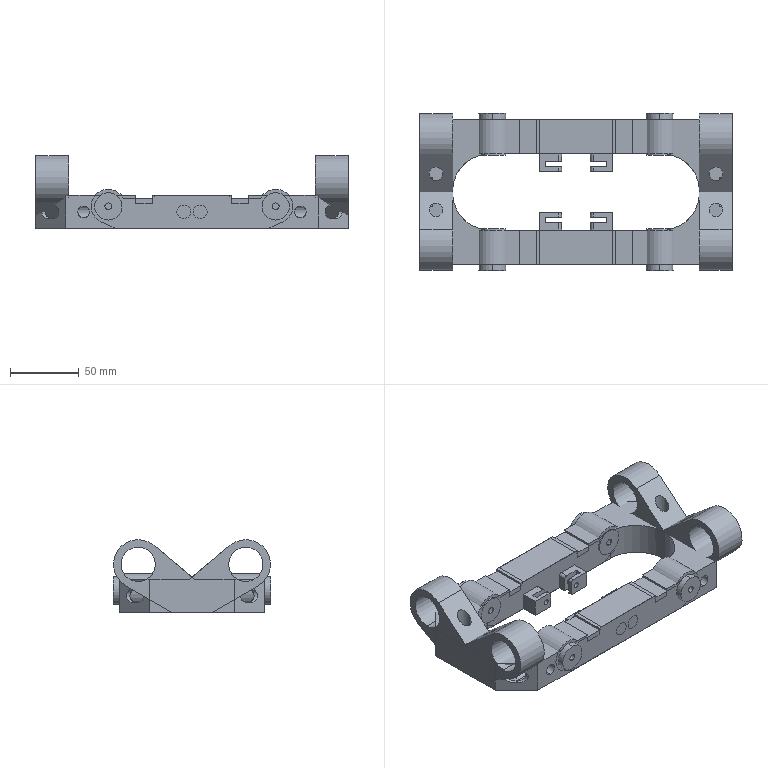NC program | Mastercam | posted with a generic post | part box 228 x 114.503 x 53 mm
Lines 3657 to 5339 of 11407:
(10 BM/BNOS |TOOL - 3|DIA. OFF. - 3|LEN. - 3|TOOL DIA. - 10.)
N7392 T3 M6
N7394 G0 G54 G90 X121.565 Y-17.392 C0. B0. S6000 M3
N7396 G43 H3 Z120.
N7398 Z31.503
N7400 Z28.503
N7402 G1 Z26.503 F600.
N7404 Y-17.366 Z26.183 F1500.
N7406 Y-17.293 Z25.869
N7408 Y-17.179 Z25.562
N7410 Y-17.03 Z25.264
N7412 Y-16.853 Z24.978
N7414 Y-16.654 Z24.707
N7416 Y-16.438 Z24.451
N7418 Y-16.214 Z24.214
N7420 X121.553 Y-16.127 Z24.127
N7422 X121.521 Y-16.044 Z24.044
N7424 X121.468 Y-15.966 Z23.966
N7426 X121.398 Y-15.892 Z23.892
N7428 X121.214 Y-15.757 Z23.757
N7430 X120.982 Y-15.644 Z23.644
N7432 X120.719 Y-15.552 Z23.552
N7434 X120.44 Y-15.484 Z23.484
N7436 X120.162 Y-15.442 Z23.442
N7438 X119.898 Y-15.428 Z23.428
N7440 X119.21
N7442 X118.024
N7444 X116.837
N7446 X115.651
N7448 X114.465
N7450 X113.278
N7452 X112.092
N7454 X110.906
N7456 X109.719
N7458 X108.533
N7460 X107.347
N7462 X106.161
N7464 X104.974
N7466 X103.788
N7468 X102.602
N7470 X101.415
N7472 X100.229
N7474 X99.043
N7476 X97.856
N7478 X96.67
N7480 X95.484
N7482 X94.297
N7484 X93.111
N7486 X91.925
N7488 X90.739
N7490 X89.552
N7492 X88.366
N7494 X87.18
N7496 X85.993
N7498 X84.807
N7500 X83.621
N7502 X82.434
N7504 X81.248
N7506 X80.062
N7508 X78.876
N7510 X77.689
N7512 X76.503
N7514 X75.317
N7516 X74.13
N7518 X72.944
N7520 X71.758
N7522 X70.571
N7524 X69.385
N7526 X68.199
N7528 X67.012
N7530 X65.826
N7532 X64.64
N7534 X63.454
N7536 X62.267
N7538 X61.081
N7540 X59.895
N7542 X58.708
N7544 X57.522
N7546 X56.336
N7548 X55.149
N7550 X53.963
N7552 X52.777
N7554 X51.591
N7556 X50.495 Y-15.429 Z23.442
N7558 X49.466 Y-15.428 Z23.489
N7560 X48.416 Z23.581
N7562 X47.37 Z23.719
N7564 X46.367 Y-15.429 Z23.898
N7566 X45.385 Z24.115
N7568 X44.38 Y-15.428 Z24.387
N7570 X43.376 Z24.707
N7572 X42.385 Z25.069
N7574 X41.432 Y-15.429 Z25.467
N7576 X40.522 Z25.895
N7578 X39.613 Y-15.428 Z26.372
N7580 X38.702 Z26.903
N7582 X37.815 Z27.474
N7584 X36.959 Z28.077
N7586 X36.165 Y-15.429 Z28.694
N7588 X35.393 Y-15.428 Z29.349
N7590 X34.619 Z30.065
N7592 X33.878 Z30.815
N7594 X33.17 Z31.597
N7596 X32.528 Y-15.429 Z32.371
N7598 X31.922 Y-15.428 Z33.173
N7600 X31.323 Z34.041
N7602 X30.762 Z34.934
N7604 X30.243 Z35.852
N7606 X29.783 Y-15.429 Z36.75
N7608 X29.365 Y-15.428 Z37.665
N7610 X28.973 Z38.639
N7612 X28.62 Z39.633
N7614 X28.312 Z40.641
N7616 X28.057 Y-15.429 Z41.633
N7618 X27.848 Z42.616
N7620 X27.679 Y-15.428 Z43.639
N7622 X27.554 Z44.686
N7624 X27.471 Z45.737
N7626 X27.441 Z46.263
N7628 X27.435 Z46.868
N7630 X27.428 Z48.149
N7632 Z49.504
N7634 Z50.86
N7636 Z52.215
N7638 Z53.57
N7640 Z54.925
N7642 Z56.28
N7644 Z57.635
N7646 Z58.99
N7648 Z60.346
N7650 Z61.701
N7652 Z62.378
N7654 X27.434 Y-15.434 Z62.61
N7656 X27.454 Y-15.454 Z62.852
N7658 X27.486 Y-15.486 Z63.101
N7660 X27.529 Y-15.529 Z63.354
N7662 X27.585 Y-15.585 Z63.607
N7664 X27.651 Y-15.651 Z63.856
N7666 X27.729 Y-15.729 Z64.098
N7668 X27.816 Y-15.816 Z64.329
N7670 X27.914 Y-15.914 Z64.546
N7672 X28.021 Y-16.021 Z64.746
N7674 X28.138 Y-16.138 Z64.924
N7676 X28.263 Y-16.263 Z65.078
N7678 X28.396 Y-16.396 Z65.204
N7680 X28.537 Y-16.537 Z65.299
N7682 X28.686 Y-16.686 Z65.358
N7684 X28.842 Y-16.842 Z65.378
N7686 X29.006 Y-17.006 Z65.387
N7688 X29.177 Y-17.177 Z65.415
N7690 X29.353 Y-17.353 Z65.46
N7692 X29.532 Y-17.532 Z65.522
N7694 X29.711 Y-17.711 Z65.6
N7696 X29.887 Y-17.887 Z65.694
N7698 X30.058 Y-18.058 Z65.804
N7700 X30.221 Y-18.221 Z65.928
N7702 X30.375 Y-18.375 Z66.066
N7704 X30.516 Y-18.516 Z66.217
N7706 X30.643 Y-18.643 Z66.382
N7708 X30.751 Y-18.751 Z66.559
N7710 X30.84 Y-18.84 Z66.747
N7712 X30.907 Y-18.907 Z66.947
N7714 X30.949 Y-18.949 Z67.158
N7716 X30.963 Y-18.963 Z67.378
N7718 G0 Z69.378
N7720 Z72.378
N7722 Z120.
N7724 X50. Y16.606
N7726 Z30.273
N7728 Z27.273
N7730 G1 Z25.273 F600.
N7732 Y16.591 Z25.081 F1500.
N7734 Y16.547 Z24.892
N7736 Y16.479 Z24.708
N7738 Y16.389 Z24.53
N7740 Y16.283 Z24.358
N7742 Y16.163 Z24.195
N7744 Y15.899 Z23.899
N7746 X50.027 Y15.798 Z23.798
N7748 X50.1 Y15.706 Z23.706
N7750 X50.211 Y15.626 Z23.626
N7752 X50.35 Y15.557 Z23.557
N7754 X50.508 Y15.502 Z23.502
N7756 X50.675 Y15.462 Z23.462
N7758 X50.842 Y15.437 Z23.437
N7760 X51. Y15.428 Z23.428
N7762 X51.733
N7764 X53.2
N7766 X54.667
N7768 X56.133
N7770 X57.6
N7772 X59.067
N7774 X60.533
N7776 X62.
N7778 X63.467
N7780 X64.933
N7782 X66.4
N7784 X67.867
N7786 X69.333
N7788 X70.8
N7790 X72.267
N7792 X73.
N7794 X73.179 Y15.423
N7796 X73.358 Y15.409
N7798 X73.536 Y15.386
N7800 X73.713 Y15.353
N7802 X73.887 Y15.311
N7804 X74.059 Y15.26
N7806 X74.228 Y15.2
N7808 X74.394 Y15.132
N7810 X74.556 Y15.054
N7812 X74.714 Y14.969
N7814 X74.867 Y14.875
N7816 X75.015 Y14.773
N7818 X75.157 Y14.664
N7820 X75.294 Y14.547
N7822 X75.424 Y14.424
N7824 X75.547 Y14.294
N7826 X75.664 Y14.157
N7828 X75.773 Y14.015
N7830 X75.875 Y13.867
N7832 X75.969 Y13.714
N7834 X76.054 Y13.556
N7836 X76.132 Y13.394
N7838 X76.2 Y13.228
N7840 X76.26 Y13.059
N7842 X76.311 Y12.887
N7844 X76.353 Y12.713
N7846 X76.386 Y12.536
N7848 X76.409 Y12.358
N7850 X76.423 Y12.179
N7852 X76.428 Y12.
N7854 Y11.25
N7856 Y9.75
N7858 Y9.428
N7860 X76.75
N7862 X78.25
N7864 X79.75
N7866 X81.25
N7868 X81.572
N7870 Y9.75
N7872 Y11.25
N7874 Y12.
N7876 X81.577 Y12.179
N7878 X81.591 Y12.358
N7880 X81.614 Y12.536
N7882 X81.647 Y12.713
N7884 X81.689 Y12.887
N7886 X81.74 Y13.059
N7888 X81.8 Y13.228
N7890 X81.868 Y13.394
N7892 X81.946 Y13.556
N7894 X82.031 Y13.714
N7896 X82.125 Y13.867
N7898 X82.227 Y14.015
N7900 X82.336 Y14.157
N7902 X82.453 Y14.294
N7904 X82.576 Y14.424
N7906 X82.706 Y14.547
N7908 X82.843 Y14.664
N7910 X82.985 Y14.773
N7912 X83.133 Y14.875
N7914 X83.286 Y14.969
N7916 X83.444 Y15.054
N7918 X83.606 Y15.132
N7920 X83.772 Y15.2
N7922 X83.941 Y15.26
N7924 X84.113 Y15.311
N7926 X84.287 Y15.353
N7928 X84.464 Y15.386
N7930 X84.642 Y15.409
N7932 X84.821 Y15.423
N7934 X85. Y15.428
N7936 X85.731
N7938 X87.193
N7940 X88.654
N7942 X90.116
N7944 X91.578
N7946 X93.04
N7948 X94.502
N7950 X95.963
N7952 X97.425
N7954 X98.887
N7956 X100.349
N7958 X101.811
N7960 X103.272
N7962 X104.734
N7964 X106.196
N7966 X107.658
N7968 X109.12
N7970 X110.581
N7972 X112.043
N7974 X113.505
N7976 X114.967
N7978 X116.429
N7980 X117.89
N7982 X119.352
N7984 X120.814
N7986 X122.276
N7988 X123.738
N7990 X125.199
N7992 X126.661
N7994 X128.123
N7996 X129.585
N7998 X131.047
N8000 X132.508
N8002 X133.97
N8004 X135.432
N8006 X136.894
N8008 X138.356
N8010 X139.817
N8012 X140.548
N8014 X140.728 Y15.423
N8016 X140.907 Y15.409
N8018 X141.084 Y15.386
N8020 X141.261 Y15.353
N8022 X141.435 Y15.311
N8024 X141.607 Y15.26
N8026 X141.777 Y15.2
N8028 X141.942 Y15.132
N8030 X142.104 Y15.054
N8032 X142.262 Y14.969
N8034 X142.415 Y14.875
N8036 X142.563 Y14.773
N8038 X142.705 Y14.664
N8040 X142.842 Y14.547
N8042 X142.972 Y14.424
N8044 X143.472 Y13.924
N8046 X143.968 Y13.428
N8048 X144.697
N8050 X146.129
N8052 X147.562
N8054 X148.994
N8056 X150.426
N8058 X151.859
N8060 X153.291
N8062 X154.724
N8064 X156.156
N8066 X157.588
N8068 X159.021
N8070 X160.453
N8072 X161.886
N8074 X162.032
N8076 X162.105
N8078 X162.178
N8080 X162.383 Y13.708 Z23.429
N8082 X162.44 Y13.779
N8084 X162.498 Y13.849
N8086 X162.555 Y13.92
N8088 X162.612 Y13.991
N8090 X162.84 Y14.274
N8092 X162.9 Y14.342
N8094 X162.96 Y14.41
N8096 X163.02 Y14.478
N8098 X163.08 Y14.546
N8100 X163.321 Y14.818
N8102 X163.826 Y15.34 Z23.428
N8104 X164.355 Y15.838
N8106 X164.906 Y16.311 Z23.429
N8108 X165.193 Y16.535
N8110 X165.264 Y16.591
N8112 X165.336 Y16.646
N8114 X165.407 Y16.702
N8116 X165.479 Y16.758
N8118 X165.775 Y16.969
N8120 X165.849 Y17.021
N8122 X165.923 Y17.074
N8124 X165.997 Y17.127
N8126 X166.071 Y17.179
N8128 X166.376 Y17.376
N8130 X166.452 Y17.426
N8132 X166.529 Y17.475
N8134 X166.681 Y17.573
N8136 X166.995 Y17.757
N8138 X167.073 Y17.802
N8140 X167.152 Y17.848
N8142 X167.309 Y17.94
N8144 X167.952 Y18.277 Z23.428
N8146 X168.544 Y18.556
N8148 X169.148 Y18.807 Z23.429
N8150 X169.319 Y18.869
N8152 X169.404 Y18.901
N8154 X169.489 Y18.932
N8156 X169.575 Y18.963
N8158 X169.66 Y18.995
N8160 X169.83 Y19.057
N8162 X170.004 Y19.112
N8164 X170.09 Y19.14
N8166 X170.177 Y19.167
N8168 X170.263 Y19.194
N8170 X170.35 Y19.222
N8172 X170.523 Y19.277
N8174 X170.611 Y19.3
N8176 X170.698 Y19.324
N8178 X170.786 Y19.347
N8180 X170.874 Y19.371
N8182 X171.225 Y19.465
N8184 X171.313 Y19.485
N8186 X171.402 Y19.504
N8188 X171.491 Y19.524
N8190 X171.579 Y19.543
N8192 X171.934 Y19.622
N8194 X172.65 Y19.746
N8196 X173.371 Y19.837 Z23.428
N8198 X174.095 Y19.894 Z23.429
N8200 X174.821 Y19.918
N8202 X175.184 Y19.914
N8204 X175.275 Y19.913
N8206 X175.366 Y19.912
N8208 X175.457 Y19.911
N8210 X175.547 Y19.91
N8212 X175.91 Y19.889
N8214 X176.001 Y19.884
N8216 X176.091 Y19.879
N8218 X176.273 Y19.869
N8220 X176.634 Y19.832
N8222 X176.724 Y19.823
N8224 X176.815 Y19.814
N8226 X176.995 Y19.795
N8228 X177.714 Y19.689
N8230 X178.357 Y19.566 Z23.428
N8232 X178.993 Y19.413 Z23.429
N8234 X179.692 Y19.213
N8236 X179.864 Y19.155
N8238 X179.95 Y19.127
N8240 X180.036 Y19.098
N8242 X180.122 Y19.069
N8244 X180.208 Y19.04
N8246 X180.381 Y18.982
N8248 X180.55 Y18.917
N8250 X180.635 Y18.884
N8252 X180.72 Y18.852
N8254 X180.804 Y18.819
N8256 X180.889 Y18.786
N8258 X181.058 Y18.721
N8260 X181.142 Y18.685
N8262 X181.225 Y18.648
N8264 X181.308 Y18.612
N8266 X181.391 Y18.575
N8268 X181.724 Y18.43
N8270 X182.376 Y18.109
N8272 X183.012 Y17.758 Z23.428
N8274 X183.631 Y17.378 Z23.429
N8276 X184.232 Y16.969
N8278 X184.523 Y16.752
N8280 X184.596 Y16.697
N8282 X184.668 Y16.643
N8284 X184.741 Y16.589
N8286 X184.814 Y16.534
N8288 X185.095 Y16.304
N8290 X185.165 Y16.247
N8292 X185.235 Y16.189
N8294 X185.376 Y16.074
N8296 X185.646 Y15.831
N8298 X185.714 Y15.771
N8300 X185.781 Y15.71
N8302 X185.916 Y15.589
N8304 X186.435 Y15.08
N8306 X186.882 Y14.601 Z23.428
N8308 X187.306 Y14.103 Z23.429
N8310 X187.753 Y13.53
N8312 X187.858 Y13.382
N8314 X187.91 Y13.308
N8316 X187.963 Y13.234
N8318 X188.016 Y13.16
N8320 X188.068 Y13.086
N8322 X188.173 Y12.938
N8324 X188.272 Y12.785
N8326 X188.321 Y12.709
N8328 X188.37 Y12.633
N8330 X188.419 Y12.557
N8332 X188.469 Y12.48
N8334 X188.567 Y12.328
N8336 X188.613 Y12.249
N8338 X188.659 Y12.171
N8340 X188.704 Y12.092
N8342 X188.75 Y12.014
N8344 X188.933 Y11.7
N8346 X188.975 Y11.62
N8348 X189.018 Y11.539
N8350 X189.06 Y11.459
N8352 X189.102 Y11.378
N8354 X189.271 Y11.057
N8356 X189.578 Y10.399 Z23.428
N8358 X189.855 Y9.727 Z23.429
N8360 X190.1 Y9.043
N8362 X190.207 Y8.696
N8364 X190.234 Y8.609
N8366 X190.26 Y8.522
N8368 X190.287 Y8.435
N8370 X190.314 Y8.348
N8372 X190.405 Y7.997
N8374 X190.428 Y7.909
N8376 X190.451 Y7.821
N8378 X190.497 Y7.645
N8380 X190.572 Y7.29
N8382 X190.591 Y7.201
N8384 X190.61 Y7.112
N8386 X190.648 Y6.935
N8388 X190.766 Y6.218
N8390 X190.846 Y5.569 Z23.428
N8392 X190.895 Y4.916 Z23.429
N8394 X190.919 Y4.19
N8396 X190.917 Y4.008
N8398 X190.916 Y3.917
N8400 X190.915 Y3.827
N8402 X190.914 Y3.736
N8404 X190.913 Y3.645
N8406 X190.91 Y3.463
N8408 X190.9 Y3.282
N8410 X190.895 Y3.191
N8412 X190.89 Y3.101
N8414 X190.884 Y3.01
N8416 X190.879 Y2.919
N8418 X190.869 Y2.738
N8420 X190.86 Y2.648
N8422 X190.85 Y2.557
N8424 X190.841 Y2.467
N8426 X190.832 Y2.377
N8428 X190.795 Y2.015
N8430 X190.782 Y1.925
N8432 X190.768 Y1.836
N8434 X190.755 Y1.746
N8436 X190.742 Y1.656
N8438 X190.689 Y1.297
N8440 X190.55 Y.583 Z23.428
N8442 X190.378 Y-.122
N8444 X190.173 Y-.819 Z23.429
N8446 X189.937 Y-1.506
N8448 X189.803 Y-1.844
N8450 X189.77 Y-1.929
N8452 X189.737 Y-2.013
N8454 X189.703 Y-2.098
N8456 X189.67 Y-2.182
N8458 X189.522 Y-2.514
N8460 X189.485 Y-2.597
N8462 X189.448 Y-2.68
N8464 X189.373 Y-2.845
N8466 X189.047 Y-3.495
N8468 X188.729 Y-4.066 Z23.428
N8470 X188.385 Y-4.623
N8472 X187.976 Y-5.224 Z23.429
N8474 X187.868 Y-5.369
N8476 X187.813 Y-5.442
N8478 X187.759 Y-5.515
N8480 X187.704 Y-5.587
N8482 X187.65 Y-5.66
N8484 X187.541 Y-5.806
N8486 X187.426 Y-5.946
N8488 X187.368 Y-6.016
N8490 X187.311 Y-6.086
N8492 X187.253 Y-6.157
N8494 X187.196 Y-6.227
N8496 X187.08 Y-6.367
N8498 X187.02 Y-6.435
N8500 X186.959 Y-6.502
N8502 X186.898 Y-6.57
N8504 X186.838 Y-6.637
N8506 X186.777 Y-6.705
N8508 X186.716 Y-6.772
N8510 X186.595 Y-6.908
N8512 X186.531 Y-6.972
N8514 X186.468 Y-7.037
N8516 X186.404 Y-7.102
N8518 X186.34 Y-7.167
N8520 X186.086 Y-7.426
N8522 X185.554 Y-7.92 Z23.428
N8524 X184.999 Y-8.39
N8526 X184.422 Y-8.832 Z23.429
N8528 X183.827 Y-9.248
N8530 X183.52 Y-9.443
N8532 X183.444 Y-9.491
N8534 X183.367 Y-9.54
N8536 X183.213 Y-9.637
N8538 X182.898 Y-9.818
N8540 X182.819 Y-9.863
N8542 X182.741 Y-9.908
N8544 X182.583 Y-9.998
N8546 X181.965 Y-10.318 Z23.428
N8548 X181.405 Y-10.584
N8550 X180.888 Y-10.819
N8552 X180.377 Y-11.052
N8554 X179.865 Y-11.284
N8556 X179.353 Y-11.517
N8558 X178.841 Y-11.749
N8560 X178.329 Y-11.982
N8562 X177.817 Y-12.214
N8564 X177.305 Y-12.447
N8566 X176.793 Y-12.679
N8568 X176.281 Y-12.912
N8570 X175.769 Y-13.145
N8572 X175.257 Y-13.377
N8574 X174.745 Y-13.61
N8576 X174.233 Y-13.842
N8578 X173.721 Y-14.075
N8580 X173.209 Y-14.307
N8582 X172.697 Y-14.54
N8584 X172.185 Y-14.772
N8586 X171.674 Y-15.005
N8588 X171.418 Y-15.121
N8590 X171.268 Y-15.185
N8592 X171.116 Y-15.241
N8594 X170.961 Y-15.29
N8596 X170.804 Y-15.332
N8598 X170.646 Y-15.367
N8600 X170.486 Y-15.393
N8602 X170.324 Y-15.413
N8604 X170.162 Y-15.424
N8606 X170. Y-15.428
N8608 X169.264
N8610 X167.791
N8612 X166.319
N8614 X164.846
N8616 X163.373
N8618 X161.901
N8620 X160.428
N8622 X158.956
N8624 X157.483
N8626 X156.01
N8628 X154.538
N8630 X153.065
N8632 X151.593
N8634 X150.12
N8636 X148.647
N8638 X147.175
N8640 X145.702
N8642 X145.198
N8644 X144.935 Y-15.442 Z23.442
N8646 X144.656 Y-15.484 Z23.484
N8648 X144.377 Y-15.552 Z23.552
N8650 X144.115 Y-15.644 Z23.644
N8652 X143.883 Y-15.757 Z23.757
N8654 X143.698 Y-15.892 Z23.892
N8656 X143.628 Y-15.966 Z23.966
N8658 X143.576 Y-16.044 Z24.044
N8660 X143.543 Y-16.127 Z24.127
N8662 X143.532 Y-16.214 Z24.214
N8664 Y-16.438 Z24.451
N8666 Y-16.654 Z24.707
N8668 Y-16.853 Z24.978
N8670 Y-17.03 Z25.264
N8672 Y-17.179 Z25.562
N8674 Y-17.293 Z25.869
N8676 Y-17.366 Z26.183
N8678 Y-17.392 Z26.503
N8680 G0 Z28.503
N8682 Z31.503
N8684 Z120.
N8686 X147.512 Y-2.84
N8688 Z46.463
N8690 Z43.463
N8692 G1 Z41.463 F600.
N8694 X147.5 Z41.175 F1500.
N8696 X147.465 Z40.888
N8698 X147.409 Z40.603
N8700 X147.334 Z40.321
N8702 X147.24 Z40.043
N8704 X147.128 Z39.768
N8706 X147.002 Z39.498
N8708 X146.861 Z39.233
N8710 X146.542 Z38.719
N8712 X146.183 Z38.23
N8714 X145.795 Z37.769
N8716 X145.39 Z37.342
N8718 X145.234 Y-2.86 Z37.186
N8720 X145.086 Y-2.919 Z37.037
N8722 X144.944 Y-3.014 Z36.896
N8724 X144.811 Y-3.139 Z36.763
N8726 X144.686 Y-3.293 Z36.638
N8728 X144.569 Y-3.472 Z36.521
N8730 X144.462 Y-3.672 Z36.414
N8732 X144.365 Y-3.889 Z36.316
N8734 X144.277 Y-4.12 Z36.229
N8736 X144.199 Y-4.362 Z36.151
N8738 X144.133 Y-4.611 Z36.085
N8740 X144.078 Y-4.864 Z36.029
N8742 X144.034 Y-5.117 Z35.986
N8744 X144.002 Y-5.366 Z35.954
N8746 X143.983 Y-5.608 Z35.934
N8748 X143.976 Y-5.84 Z35.928
N8750 Y-7.139
N8752 Y-8.528
N8754 Y-9.917
N8756 Y-11.306
N8758 Y-12.
N8760 X143.971 Y-12.179
N8762 X143.957 Y-12.358
N8764 X143.934 Y-12.536
N8766 X143.901 Y-12.713
N8768 X143.859 Y-12.887
N8770 X143.808 Y-13.059
N8772 X143.748 Y-13.228
N8774 X143.68 Y-13.394
N8776 X143.602 Y-13.556
N8778 X143.517 Y-13.714
N8780 X143.423 Y-13.867
N8782 X143.321 Y-14.015
N8784 X143.212 Y-14.157
N8786 X143.096 Y-14.294
N8788 X142.972 Y-14.424
N8790 X142.842 Y-14.547
N8792 X142.705 Y-14.664
N8794 X142.563 Y-14.773
N8796 X142.415 Y-14.875
N8798 X142.262 Y-14.969
N8800 X142.104 Y-15.054
N8802 X141.942 Y-15.132
N8804 X141.777 Y-15.2
N8806 X141.607 Y-15.26
N8808 X141.435 Y-15.311
N8810 X141.261 Y-15.353
N8812 X141.084 Y-15.386
N8814 X140.907 Y-15.409
N8816 X140.728 Y-15.423
N8818 X140.548 Y-15.428
N8820 X139.821
N8822 X138.366
N8824 X136.912
N8826 X135.457
N8828 X134.003
N8830 X132.548
N8832 X131.094
N8834 X129.639
N8836 X128.185
N8838 X126.73
N8840 X125.275
N8842 X124.548
N8844 X124.369 Y-15.423
N8846 X124.19 Y-15.409
N8848 X124.012 Y-15.386
N8850 X123.836 Y-15.353
N8852 X123.661 Y-15.311
N8854 X123.489 Y-15.26
N8856 X123.32 Y-15.2
N8858 X123.154 Y-15.132
N8860 X122.992 Y-15.054
N8862 X122.834 Y-14.969
N8864 X122.681 Y-14.875
N8866 X122.533 Y-14.773
N8868 X122.391 Y-14.664
N8870 X122.255 Y-14.547
N8872 X122.124 Y-14.424
N8874 X122.001 Y-14.294
N8876 X121.884 Y-14.157
N8878 X121.775 Y-14.015
N8880 X121.673 Y-13.867
N8882 X121.58 Y-13.714
N8884 X121.494 Y-13.556
N8886 X121.417 Y-13.394
N8888 X121.348 Y-13.228
N8890 X121.288 Y-13.059
N8892 X121.237 Y-12.887
N8894 X121.195 Y-12.713
N8896 X121.163 Y-12.536
N8898 X121.139 Y-12.358
N8900 X121.125 Y-12.179
N8902 X121.12 Y-12.
N8904 Y-10.5
N8906 Y-9.75
N8908 Y-8.25
N8910 Y-6.75
N8912 Y-5.25
N8914 Y-3.75
N8916 Y-3.
N8918 X121.125 Y-1.321
N8920 X121.148 Y-1.169 Z35.936
N8922 X121.159 Y-1.094 Z35.94
N8924 X121.171 Y-1.018 Z35.945
N8926 X121.182 Y-.942 Z35.949
N8928 X121.194 Y-.866 Z35.953
N8930 X121.207 Y-.79 Z35.956
N8932 X121.22 Y-.715 Z35.958
N8934 X121.234 Y-.639 Z35.959
N8936 X121.249 Y-.564 Z35.96
N8938 X121.264 Y-.488 Z35.961
N8940 X121.279 Y-.413 Z35.962
N8942 X121.309 Y-.318 Z35.972
N8944 X121.34 Y-.224 Z35.982
N8946 X121.372 Y-.13 Z35.989
N8948 X121.404 Y-.036 Z35.997
N8950 X121.422 Y.011 Z35.999
N8952 X121.44 Y.058 Z36.002
N8954 X121.457 Y.105 Z36.004
N8956 X121.475 Y.151 Z36.007
N8958 X121.493 Y.198 Z36.009
N8960 X121.511 Y.245 Z36.011
N8962 X121.529 Y.292 Z36.013
N8964 X121.547 Y.339 Z36.015
N8966 X121.565 Y.385 Z36.017
N8968 X121.584 Y.432 Z36.019
N8970 X121.603 Y.479
N8972 X121.622 Y.525 Z36.02
N8974 X121.642 Y.572
N8976 X121.662 Y.618 Z36.021
N8978 X121.682 Y.664 Z36.02
N8980 X121.703 Y.71 Z36.019
N8982 X121.724 Y.755 Z36.018
N8984 X121.745 Y.801 Z36.017
N8986 X121.765 Y.847 Z36.016
N8988 X121.786 Y.892 Z36.015
N8990 X121.808 Y.938 Z36.014
N8992 X121.829 Y.983 Z36.012
N8994 X121.85 Y1.029 Z36.01
N8996 X121.871 Y1.074 Z36.009
N8998 X121.916 Y1.163 Z36.003
N9000 X121.96 Y1.252 Z35.997
N9002 X122.007 Y1.34 Z35.989
N9004 X122.054 Y1.427 Z35.98
N9006 X122.111 Y1.496 Z35.989
N9008 X122.168 Y1.565 Z35.997
N9010 X122.226 Y1.634 Z36.005
N9012 X122.283 Y1.703 Z36.013
N9014 X122.343 Y1.77 Z36.018
N9016 X122.403 Y1.838 Z36.023
N9018 X122.465 Y1.905 Z36.027
N9020 X122.527 Y1.972 Z36.03
N9022 X122.589 Y2.038 Z36.033
N9024 X122.651 Y2.105 Z36.035
N9026 X122.715 Y2.17 Z36.037
N9028 X122.778 Y2.236 Z36.038
N9030 X122.843 Y2.3 Z36.037
N9032 X122.908 Y2.364 Z36.036
N9034 X122.974 Y2.427 Z36.033
N9036 X123.04 Y2.489 Z36.03
N9038 X123.106 Y2.552 Z36.027
N9040 X123.172 Y2.614 Z36.023
N9042 X123.24 Y2.675 Z36.018
N9044 X123.307 Y2.735 Z36.013
N9046 X123.375 Y2.794 Z36.005
N9048 X123.443 Y2.852 Z35.998
N9050 X123.512 Y2.909 Z35.989
N9052 X123.58 Y2.967 Z35.98
N9054 X123.656 Y3.007 Z35.988
N9056 X123.731 Y3.048 Z35.997
N9058 X123.808 Y3.087 Z36.003
N9060 X123.885 Y3.126 Z36.01
N9062 X123.963 Y3.164 Z36.014
N9064 X124.041 Y3.202 Z36.018
N9066 X124.12 Y3.238 Z36.021
N9068 X124.199 Y3.274 Z36.023
N9070 X124.279 Y3.31 Z36.025
N9072 X124.358 Y3.346 Z36.027
N9074 X124.438 Y3.38 Z36.028
N9076 X124.518 Y3.415 Z36.029
N9078 X124.599 Y3.448 Z36.027
N9080 X124.68 Y3.48 Z36.026
N9082 X124.761 Y3.511 Z36.022
N9084 X124.843 Y3.542 Z36.019
N9086 X124.924 Y3.573 Z36.016
N9088 X125.005 Y3.604 Z36.012
N9090 X125.087 Y3.633 Z36.007
N9092 X125.168 Y3.662 Z36.002
N9094 X125.25 Y3.689 Z35.995
N9096 X125.331 Y3.716 Z35.987
N9098 X125.413 Y3.742 Z35.979
N9100 X125.495 Y3.767 Z35.97
N9102 X125.553 Y3.777 Z35.971
N9104 X125.611 Y3.787 Z35.973
N9106 X125.669 Y3.796 Z35.974
N9108 X125.727 Y3.806 Z35.976
N9110 X125.785 Y3.815
N9112 X125.843 Y3.823
N9114 X125.902 Y3.831 Z35.975
N9116 X125.96 Y3.838 Z35.974
N9118 X126.018 Y3.845 Z35.972
N9120 X126.077 Y3.851 Z35.971
N9122 X126.135 Y3.858 Z35.969
N9124 X126.194 Y3.864 Z35.967
N9126 X126.252 Y3.87 Z35.964
N9128 X126.311 Y3.876 Z35.962
N9130 X126.369 Y3.882 Z35.96
N9132 X126.428 Y3.888 Z35.957
N9134 X126.486 Y3.893 Z35.954
N9136 X126.545 Y3.897 Z35.95
N9138 X126.662 Y3.907 Z35.943
N9140 X126.895 Y3.926 Z35.929
N9142 X127.696 Y3.928 Z35.928
N9144 X128.475
N9146 X129.254
N9148 X130.033
N9150 X130.811
N9152 X131.59
N9154 X132.369
N9156 X133.148
N9158 X133.927
N9160 X134.706
N9162 X135.485
N9164 X136.264
N9166 X137.043
N9168 X137.822
N9170 X138.601
N9172 X139.38
N9174 X140.159
N9176 X140.548
N9178 X140.728 Y3.923
N9180 X140.907 Y3.909
N9182 X141.084 Y3.886
N9184 X141.261 Y3.853
N9186 X141.435 Y3.811
N9188 X141.607 Y3.76
N9190 X141.777 Y3.7
N9192 X141.942 Y3.632
N9194 X142.104 Y3.554
N9196 X142.262 Y3.469
N9198 X142.415 Y3.375
N9200 X142.563 Y3.273
N9202 X142.705 Y3.164
N9204 X142.842 Y3.047
N9206 X142.972 Y2.924
N9208 X143.096 Y2.794
N9210 X143.212 Y2.657
N9212 X143.321 Y2.515
N9214 X143.423 Y2.367
N9216 X143.517 Y2.214
N9218 X143.602 Y2.056
N9220 X143.68 Y1.894
N9222 X143.748 Y1.728
N9224 X143.808 Y1.559
N9226 X143.859 Y1.387
N9228 X143.901 Y1.213
N9230 X143.934 Y1.036
N9232 X143.957 Y.858
N9234 X143.971 Y.679
N9236 X143.976 Y.5
N9238 Y-.194
N9240 Y-1.583
N9242 Y-2.972
N9244 Y-4.361
N9246 Y-5.75
N9248 Y-5.84
N9250 X143.983 Y-6.071 Z35.934
N9252 X144.002 Y-6.314 Z35.954
N9254 X144.034 Y-6.563 Z35.986
N9256 X144.078 Y-6.815 Z36.029
N9258 X144.133 Y-7.068 Z36.085
N9260 X144.199 Y-7.317 Z36.151
N9262 X144.277 Y-7.559 Z36.229
N9264 X144.365 Y-7.79 Z36.316
N9266 X144.462 Y-8.008 Z36.414
N9268 X144.569 Y-8.207 Z36.521
N9270 X144.686 Y-8.386 Z36.638
N9272 X144.811 Y-8.54 Z36.763
N9274 X144.944 Y-8.666 Z36.896
N9276 X145.086 Y-8.76 Z37.037
N9278 X145.234 Y-8.819 Z37.186
N9280 X145.39 Y-8.84 Z37.342
N9282 X145.795 Z37.769
N9284 X146.183 Z38.23
N9286 X146.542 Z38.719
N9288 X146.861 Z39.233
N9290 X147.002 Z39.498
N9292 X147.128 Z39.768
N9294 X147.24 Z40.043
N9296 X147.334 Z40.321
N9298 X147.409 Z40.603
N9300 X147.465 Z40.888
N9302 X147.5 Z41.175
N9304 X147.512 Z41.463
N9306 G0 Z43.463
N9308 Z46.463
N9310 Z120.
N9312 X30.918 Y47.863
N9314 Z90.754
N9316 Z87.754
N9318 G1 Z85.754 F600.
N9320 X30.904 Y47.849 Z85.534 F1500.
N9322 X30.862 Y47.807 Z85.324
N9324 X30.795 Y47.74 Z85.125
N9326 X30.706 Y47.651 Z84.937
N9328 X30.597 Y47.542 Z84.761
N9330 X30.471 Y47.416 Z84.598
N9332 X30.329 Y47.274 Z84.447
N9334 X30.175 Y47.121 Z84.311
N9336 X30.012 Y46.957 Z84.188
N9338 X29.84 Y46.786 Z84.08
N9340 X29.664 Y46.61 Z83.987
N9342 X29.486 Y46.431 Z83.91
N9344 X29.307 Y46.253 Z83.849
N9346 X29.131 Y46.077 Z83.806
N9348 X28.96 Y45.906 Z83.78
N9350 X28.797 Y45.743 Z83.772
N9352 X28.643 Y45.589 Z83.794
N9354 X28.496 Y45.443 Z83.855
N9356 X28.357 Y45.305 Z83.951
N9358 X28.226 Y45.176 Z84.079
N9360 X28.103 Y45.055 Z84.234
N9362 X27.99 Y44.944 Z84.415
N9364 X27.885 Y44.843 Z84.616
N9366 X27.79 Y44.751 Z84.835
N9368 X27.706 Y44.669 Z85.067
N9370 X27.632 Y44.598 Z85.31
N9372 X27.568 Y44.538 Z85.56
N9374 X27.516 Y44.489 Z85.812
N9376 X27.476 Y44.452 Z86.065
N9378 X27.447 Y44.427 Z86.313
N9380 X27.431 Y44.414 Z86.553
N9382 X27.428 Z86.783
N9384 X27.429 Y44.416 Z86.858
N9386 X27.428 Z86.932
N9388 Y44.417 Z87.007
N9390 Y44.418 Z87.082
N9392 Y44.422 Z87.381
N9394 Z86.982
N9396 X27.431 Y44.417 Z86.583
N9398 X27.432 Y44.414 Z86.384
N9400 X27.433 Y44.413 Z86.284
N9402 Y44.412 Z86.184
N9404 X27.428 Y44.414 Z86.783
N9406 Y44.422 Z87.381
N9408 Y44.398 Z87.911
N9410 X27.431 Y44.365 Z88.439
N9412 Y44.36 Z88.506
N9414 Y44.355 Z88.572
N9416 X27.43 Y44.35 Z88.638
N9418 Y44.345 Z88.704
N9420 X27.429 Y44.326 Z88.968
N9422 X27.43 Y44.312 Z89.1
N9424 Y44.305 Z89.166
N9426 X27.431 Y44.298 Z89.231
N9428 Y44.29 Z89.297
N9430 Y44.282 Z89.363
N9432 X27.43 Y44.274 Z89.429
N9434 Y44.267 Z89.495
N9436 Y44.251 Z89.626
N9438 Y44.243 Z89.692
N9440 X27.429 Y44.235 Z89.758
N9442 Y44.227 Z89.823
N9444 Y44.22 Z89.889
N9446 X27.428 Y44.204 Z90.021
N9448 X27.43 Y44.118 Z90.544
N9450 Y44.107 Z90.609
N9452 Y44.096 Z90.674
N9454 Y44.085 Z90.74
N9456 X27.429 Y44.074 Z90.805
N9458 Y44.063 Z90.87
N9460 Y44.052 Z90.935
N9462 X27.428 Y44.029 Z91.066
N9464 X27.429 Y44. Z91.2
N9466 Y43.985 Z91.267
N9468 X27.43 Y43.971 Z91.334
N9470 Y43.957 Z91.401
N9472 X27.431 Y43.942 Z91.469
N9474 Y43.927 Z91.536
N9476 Y43.912 Z91.602
N9478 Y43.897 Z91.669
N9480 X27.43 Y43.882 Z91.736
N9482 Y43.852 Z91.87
N9484 X27.429 Y43.792 Z92.138
N9486 X27.43 Y43.773 Z92.206
N9488 Y43.755 Z92.273
N9490 Y43.737 Z92.341
N9492 Y43.718 Z92.408
N9494 Y43.7 Z92.476
N9496 Y43.682 Z92.543
N9498 X27.431 Y43.664 Z92.611
N9500 Y43.645 Z92.679
N9502 Y43.627 Z92.746
N9504 Y43.608 Z92.814
N9506 Y43.59 Z92.881
N9508 Y43.571 Z92.949
N9510 X27.43 Y43.553 Z93.016
N9512 Y43.534 Z93.083
N9514 X27.429 Y43.496 Z93.218
N9516 X27.43 Y43.412 Z93.475
N9518 Y43.391 Z93.539
N9520 Y43.37 Z93.603
N9522 X27.431 Y43.349 Z93.668
N9524 Y43.328 Z93.732
N9526 Y43.306 Z93.796
N9528 X27.43 Y43.285 Z93.86
N9530 Y43.242 Z93.988
N9532 X27.428 Y43.156 Z94.244
N9534 X27.429 Y43.132 Z94.306
N9536 Y43.108 Z94.368
N9538 Y43.084 Z94.43
N9540 Y43.061 Z94.491
N9542 Y43.037 Z94.553
N9544 X27.43 Y43.013 Z94.615
N9546 Y42.989 Z94.677
N9548 Y42.965 Z94.738
N9550 Y42.941 Z94.8
N9552 Y42.917 Z94.862
N9554 X27.431 Y42.893 Z94.924
N9556 Y42.869 Z94.986
N9558 X27.43 Y42.845 Z95.047
N9560 Y42.82 Z95.109
N9562 X27.429 Y42.771 Z95.232
N9564 X27.43 Y42.665 Z95.474
N9566 X27.431 Y42.638 Z95.535
N9568 Y42.612 Z95.596
N9570 Y42.585 Z95.656
N9572 X27.432 Y42.559 Z95.717
N9574 X27.431 Y42.531 Z95.778
N9576 Y42.504 Z95.838
N9578 X27.43 Y42.45 Z95.959
N9580 X27.428 Y42.341 Z96.2
N9582 X27.429 Y42.282 Z96.319
N9584 X27.43 Y42.252 Z96.378
N9586 Y42.223 Z96.437
N9588 Y42.193 Z96.496
N9590 Y42.163 Z96.555
N9592 Y42.133 Z96.615
N9594 Y42.103 Z96.674
N9596 Y42.073 Z96.733
N9598 Y42.043 Z96.792
N9600 Y42.013 Z96.851
N9602 X27.429 Y41.982 Z96.91
N9604 Y41.952 Z96.969
N9606 Y41.922 Z97.028
N9608 Y41.892 Z97.087
N9610 X27.428 Y41.862 Z97.146
N9612 X27.43 Y41.732 Z97.376
N9614 Y41.666 Z97.492
N9616 X27.431 Y41.634 Z97.549
N9618 Y41.601 Z97.607
N9620 Y41.568 Z97.664
N9622 X27.432 Y41.536 Z97.722
N9624 X27.431 Y41.502 Z97.779
N9626 X27.43 Y41.469 Z97.836
N9628 Y41.435 Z97.894
N9630 X27.429 Y41.402 Z97.951
N9632 Y41.336 Z98.066
N9634 X27.43 Y41.266 Z98.178
N9636 Y41.231 Z98.234
N9638 X27.431 Y41.196 Z98.29
N9640 Y41.16 Z98.346
N9642 Y41.124 Z98.402
N9644 Y41.089 Z98.458
N9646 Y41.053 Z98.514
N9648 X27.43 Y40.982 Z98.625
N9650 Y40.946 Z98.681
N9652 Y40.91 Z98.737
N9654 X27.429 Y40.874 Z98.793
N9656 Y40.839 Z98.848
N9658 X27.428 Y40.767 Z98.96
N9660 X27.429 Y40.729 Z99.014
N9662 Y40.691 Z99.068
N9664 Y40.615 Z99.177
N9666 X27.43 Y40.538 Z99.285
N9668 Y40.462 Z99.393
N9670 Y40.424 Z99.447
N9672 Y40.386 Z99.501
N9674 Y40.347 Z99.555
N9676 Y40.309 Z99.609
N9678 X27.428 Y40.154 Z99.825
N9680 X27.429 Y40.07 Z99.932
N9682 Y40.028 Z99.986
N9684 X27.43 Y39.986 Z100.04
N9686 Y39.943 Z100.094
N9688 Y39.901 Z100.148
N9690 X27.431 Y39.859 Z100.202
N9692 Y39.817 Z100.256
N9694 Y39.774 Z100.309
N9696 Y39.731 Z100.363
N9698 X27.43 Y39.646 Z100.47
N9700 X27.429 Y39.475 Z100.684
N9702 X27.43 Y39.429 Z100.737
N9704 Y39.383 Z100.79
N9706 Y39.337 Z100.843
N9708 Y39.291 Z100.896
N9710 Y39.246 Z100.948
N9712 Y39.2 Z101.001
N9714 X27.431 Y39.154 Z101.054
N9716 Y39.108 Z101.107
N9718 Y39.062 Z101.16
N9720 Y39.016 Z101.212
N9722 Y38.97 Z101.265
N9724 Y38.924 Z101.318
N9726 Y38.878 Z101.37
N9728 X27.43 Y38.831 Z101.423
N9730 X27.429 Y38.738 Z101.527
N9732 X27.43 Y38.55 Z101.723
N9734 Y38.504 Z101.771
N9736 X27.431 Y38.457 Z101.82
N9738 Y38.41 Z101.869
N9740 Y38.363 Z101.918
N9742 Y38.315 Z101.966
N9744 X27.43 Y38.268 Z102.014
N9746 Y38.173 Z102.111
N9748 X27.428 Y37.984 Z102.305
N9750 X27.429 Y37.935 Z102.35
N9752 Y37.887 Z102.395
N9754 Y37.839 Z102.44
N9756 Y37.79 Z102.486
N9758 X27.43 Y37.742 Z102.531
N9760 Y37.693 Z102.576
N9762 Y37.645 Z102.621
N9764 Y37.596 Z102.666
N9766 Y37.548 Z102.711
N9768 Y37.499 Z102.757
N9770 Y37.451 Z102.802
N9772 Y37.402 Z102.847
N9774 Y37.354 Z102.892
N9776 X27.429 Y37.305 Z102.936
N9778 Y37.256 Z102.981
N9780 Y37.207 Z103.026
N9782 X27.432 Y36.804 Z103.37
N9784 X27.431 Y36.753 Z103.412
N9786 Y36.702 Z103.455
N9788 X27.43 Y36.652 Z103.497
N9790 Y36.601 Z103.54
N9792 X27.429 Y36.397 Z103.709
N9794 X27.43 Y36.293 Z103.791
N9796 Y36.24 Z103.831
N9798 X27.431 Y36.188 Z103.872
N9800 Y36.135 Z103.912
N9802 Y36.082 Z103.952
N9804 X27.43 Y36.03 Z103.992
N9806 Y35.977 Z104.032
N9808 Y35.924 Z104.072
N9810 Y35.871 Z104.112
N9812 Y35.818 Z104.152
N9814 X27.429 Y35.766 Z104.192
N9816 Y35.713 Z104.232
N9818 Y35.66 Z104.272
N9820 Y35.607 Z104.312
N9822 X27.428 Y35.554 Z104.352
N9824 X27.43 Y35.336 Z104.503
N9826 Y35.282 Z104.54
N9828 Y35.227 Z104.578
N9830 X27.431 Y35.173 Z104.616
N9832 Y35.119 Z104.653
N9834 Y35.064 Z104.691
N9836 X27.432 Y35.01 Z104.729
N9838 X27.431 Y34.955 Z104.766
N9840 Y34.9 Z104.803
N9842 X27.43 Y34.845 Z104.84
N9844 Y34.79 Z104.877
N9846 X27.429 Y34.68 Z104.951
N9848 Y34.568 Z105.021
N9850 X27.43 Y34.511 Z105.056
N9852 Y34.455 Z105.091
N9854 X27.431 Y34.399 Z105.127
N9856 X27.432 Y34.343 Z105.162
N9858 X27.431 Y34.287 Z105.197
N9860 Y34.23 Z105.231
N9862 Y34.174 Z105.266
N9864 X27.43 Y34.117 Z105.3
N9866 Y34.004 Z105.369
N9868 X27.429 Y33.778 Z105.507
N9870 Y33.72 Z105.54
N9872 Y33.662 Z105.572
N9874 Y33.604 Z105.604
N9876 Y33.547 Z105.636
N9878 Y33.489 Z105.668
N9880 X27.43 Y33.431 Z105.7
N9882 Y33.373 Z105.732
N9884 Y33.315 Z105.764
N9886 Y33.257 Z105.796
N9888 Y33.199 Z105.828
N9890 Y33.141 Z105.86
N9892 Y33.083 Z105.892
N9894 Y33.025 Z105.924
N9896 X27.429 Y32.966 Z105.956
N9898 X27.428 Y32.85 Z106.019
N9900 X27.43 Y32.612 Z106.136
N9902 Y32.553 Z106.165
N9904 Y32.493 Z106.194
N9906 X27.431 Y32.434 Z106.224
N9908 Y32.375 Z106.253
N9910 Y32.315 Z106.281
N9912 Y32.255 Z106.31
N9914 X27.43 Y32.136 Z106.367
N9916 X27.429 Y31.897 Z106.482
N9918 Y31.833 Z106.51
N9920 X27.43 Y31.769 Z106.537
N9922 Y31.705 Z106.565
N9924 Y31.642 Z106.593
N9926 Y31.578 Z106.62
N9928 Y31.513 Z106.647
N9930 Y31.449 Z106.674
N9932 Y31.385 Z106.702
N9934 Y31.321 Z106.729
N9936 X27.431 Y31.257 Z106.756
N9938 Y31.193 Z106.783
N9940 Y31.129 Z106.811
N9942 X27.43 Y31.065 Z106.838
N9944 Y31.001 Z106.865
N9946 X27.429 Y30.873 Z106.918
N9948 X27.431 Y30.61 Z107.016
N9950 Y30.479 Z107.064
N9952 Y30.414 Z107.089
N9954 X27.432 Y30.348 Z107.113
N9956 X27.431 Y30.282 Z107.137
N9958 Y30.216 Z107.161
N9960 X27.43 Y30.151 Z107.184
N9962 Y30.085 Z107.208
N9964 X27.429 Y29.821 Z107.303
N9966 Y29.694 Z107.343
N9968 X27.43 Y29.631 Z107.363
N9970 Y29.567 Z107.383
N9972 Y29.503 Z107.402
N9974 Y29.44 Z107.422
N9976 Y29.376 Z107.441
N9978 Y29.312 Z107.461
N9980 Y29.249 Z107.48
N9982 Y29.185 Z107.5
N9984 X27.429 Y29.121 Z107.519
N9986 Y29.057 Z107.538
N9988 Y28.994 Z107.558
N9990 X27.43 Y28.93 Z107.578
N9992 X27.429 Y28.866 Z107.597
N9994 Y28.802 Z107.616
N9996 X27.431 Y28.289 Z107.749
N9998 Y28.225 Z107.766
N100 Y28.161 Z107.782
N102 Y28.097 Z107.798
N104 X27.43 Y28.032 Z107.814
N106 X27.429 Y27.968 Z107.83
N108 Y27.904 Z107.846
N110 Y27.775 Z107.878
N112 X27.431 Y27.516 Z107.933
N114 Y27.451 Z107.946
N116 X27.43 Y27.386 Z107.959
N118 Y27.321 Z107.972
N120 Y27.256 Z107.985
N122 Y27.191 Z107.998
N124 Y27.126 Z108.011
N126 Y27.062 Z108.024
N128 X27.429 Y26.997 Z108.037
N130 X27.428 Y26.737 Z108.089
N132 X27.429 Y26.671 Z108.099
N134 Y26.606 Z108.109
N136 Y26.54 Z108.119
N138 X27.43 Y26.475 Z108.129
N140 Y26.409 Z108.139
N142 Y26.344 Z108.15
N144 Y26.279 Z108.16
N146 X27.431 Y26.213 Z108.17
N148 Y26.148 Z108.18
N150 Y26.082 Z108.19
N152 Y26.017 Z108.2
N154 Y25.951 Z108.21
N156 X27.43 Y25.886 Z108.219
N158 Y25.82 Z108.228
N160 X27.429 Y25.689 Z108.247
N162 Y25.557 Z108.261
N164 X27.43 Y25.491 Z108.268
N166 Y25.425 Z108.275
N168 X27.431 Y25.36 Z108.283
N170 X27.432 Y25.294 Z108.29
N172 Y25.228 Z108.297
N174 Y25.162 Z108.303
N176 X27.429 Y24.634 Z108.354
N178 Y24.568 Z108.358
N180 Y24.502 Z108.362
N182 X27.43 Y24.436 Z108.366
N184 Y24.37 Z108.37
N186 Y24.304 Z108.373
N188 Y24.238 Z108.377
N190 Y24.172 Z108.38
N192 Y24.105 Z108.384
N194 Y24.039 Z108.387
N196 Y23.973 Z108.391
N198 Y23.907 Z108.394
N200 Y23.841 Z108.398
N202 Y23.775 Z108.401
N204 X27.429 Y23.709 Z108.404
N206 Y23.642 Z108.407
N208 X27.428 Y23.576 Z108.41
N210 X27.43 Y23.311 Z108.412
N212 Y23.245
N214 X27.431 Y23.179 Z108.413
N216 Y23.113
N218 Y23.046 Z108.414
N220 Y22.98 Z108.413
N222 Y22.914
N224 X27.43 Y22.848
N226 Y22.781
N228 X27.429 Y22.516 Z108.412
N230 X27.43 Y22.378 Z108.406
N232 Y22.308 Z108.403
N234 X27.431 Y22.239 Z108.401
N236 Y22.17 Z108.397
N238 Y22.1 Z108.394
N240 Y22.031 Z108.39
N242 Y21.962 Z108.387
N244 X27.43 Y21.892 Z108.383
N246 Y21.823 Z108.38
N248 Y21.754 Z108.376
N250 Y21.684 Z108.372
N252 Y21.615 Z108.369
N254 Y21.546 Z108.365
N256 Y21.476 Z108.362
N258 Y21.407 Z108.358
N260 X27.432 Y20.85 Z108.305
N262 Y20.78 Z108.298
N264 Y20.71 Z108.291
N266 X27.431 Y20.641 Z108.284
N268 X27.43 Y20.571 Z108.276
N270 X27.429 Y20.293 Z108.247
N272 X27.43 Y20.029 Z108.208
N274 Y19.963 Z108.198
N276 Y19.897 Z108.187
N278 Y19.831 Z108.177
N280 Y19.765 Z108.167
N282 Y19.699 Z108.157
N284 Y19.633 Z108.146
N286 X27.429 Y19.567 Z108.136
N288 Y19.501 Z108.126
N290 Y19.435 Z108.115
N292 Y19.369 Z108.105
N294 Y19.303 Z108.095
N296 Y19.237 Z108.084
N298 X27.431 Y18.717 Z107.98
N300 Y18.652 Z107.967
N302 Y18.587 Z107.954
N304 Y18.523 Z107.94
N306 X27.43 Y18.458 Z107.927
N308 X27.429 Y18.199 Z107.872
N310 Y18.07 Z107.84
N312 Y18.006 Z107.823
N314 X27.43 Y17.942 Z107.807
N316 Y17.877 Z107.792
N318 X27.431 Y17.813 Z107.776
N320 Y17.749 Z107.759
N322 Y17.685 Z107.743
N324 X27.43 Y17.621 Z107.726
N326 Y17.557 Z107.709
N328 Y17.492 Z107.693
N330 Y17.428 Z107.676
N332 X27.428 Y17.172 Z107.609
N334 X27.429 Y17.109 Z107.59
N336 Y17.045 Z107.57
N338 Y16.982 Z107.551
N340 Y16.919 Z107.531
N342 X27.43 Y16.855 Z107.512
N344 Y16.792 Z107.493
N346 Y16.729 Z107.473
N348 Y16.665 Z107.454
N350 Y16.602 Z107.434
N352 X27.431 Y16.539 Z107.415
N354 Y16.475 Z107.395
N356 Y16.412 Z107.376
N358 X27.43 Y16.349 Z107.355
N360 Y16.286 Z107.335
N362 X27.429 Y16.16 Z107.295
N364 X27.43 Y15.91 Z107.205
N366 X27.431 Y15.848 Z107.183
N368 Y15.786 Z107.161
N370 Y15.723 Z107.139
N372 X27.432 Y15.661 Z107.116
N374 X27.431 Y15.599 Z107.093
N376 Y15.537 Z107.07
N378 X27.43 Y15.413 Z107.024
N380 X27.429 Y15.164 Z106.931
N382 Y15.103 Z106.906
N384 X27.43 Y15.042 Z106.881
N386 Y14.98 Z106.856
N388 X27.431 Y14.919 Z106.831
N390 Y14.858 Z106.805
N392 X27.43 Y14.797 Z106.779
N394 Y14.736 Z106.753
N396 Y14.675 Z106.728
N398 Y14.614 Z106.702
N400 Y14.553 Z106.676
N402 Y14.492 Z106.65
N404 X27.429 Y14.431 Z106.624
N406 Y14.37 Z106.598
N408 Y14.309 Z106.572
N410 Y14.248 Z106.546
N412 X27.428 Y14.187 Z106.52
N414 X27.43 Y13.948 Z106.406
N416 Y13.888 Z106.378
N418 Y13.829 Z106.35
N420 X27.431 Y13.769 Z106.321
N422 Y13.709 Z106.293
N424 Y13.649 Z106.264
N426 Y13.59 Z106.235
N428 X27.43 Y13.53 Z106.206
N430 Y13.471 Z106.176
N432 X27.429 Y13.411 Z106.147
N434 Y13.352 Z106.118
N436 Y13.233 Z106.06
N438 X27.43 Y12.999 Z105.936
N440 Y12.941 Z105.904
N442 Y12.883 Z105.872
N444 Y12.825 Z105.841
N446 Y12.766 Z105.809
N448 X27.429 Y12.534 Z105.682
N450 Y12.476 Z105.65
N452 Y12.418 Z105.618
N454 Y12.36 Z105.586
N456 Y12.302 Z105.554
N458 X27.43 Y12.062 Z105.409
N460 X27.431 Y11.823 Z105.264
N462 Y11.763 Z105.228
N464 X27.432 Y11.703 Z105.192
N466 X27.431 Y11.644 Z105.154
N468 X27.43 Y11.585 Z105.117
N470 Y11.525 Z105.081
N472 Y11.466 Z105.044
N474 X27.429 Y11.346 Z104.971
N476 X27.43 Y11.115 Z104.813
N478 X27.431 Y11.057 Z104.774
N480 X27.432 Y10.999 Z104.735
N482 X27.431 Y10.941 Z104.695
N484 Y10.884 Z104.655
N486 Y10.826 Z104.615
N488 X27.43 Y10.769 Z104.576
N490 Y10.654 Z104.496
N492 X27.429 Y10.424 Z104.337
N494 Y10.371 Z104.297
N496 Y10.318 Z104.257
N498 Y10.265 Z104.216
N500 Y10.213 Z104.176
N502 X27.43 Y10.002 Z104.016
N504 Y9.949 Z103.976
N506 Y9.896 Z103.936
N508 X27.431 Y9.844 Z103.895
N510 Y9.791 Z103.855
N512 X27.429 Y9.582 Z103.693
N514 X27.43 Y9.379 Z103.523
N516 Y9.328 Z103.48
N518 Y9.277 Z103.438
N520 X27.431 Y9.226 Z103.395
N522 Y9.175 Z103.353
N524 Y9.125 Z103.31
N526 X27.43 Y9.075 Z103.267
N528 Y9.024 Z103.224
N530 Y8.974 Z103.181
N532 X27.428 Y8.772 Z103.009
N534 X27.429 Y8.724 Z102.964
N536 Y8.675 Z102.919
N538 X27.43 Y8.626 Z102.874
N540 X27.429 Y8.578 Z102.828
N542 X27.43 Y8.53 Z102.783
N544 Y8.481 Z102.738
N546 Y8.433 Z102.693
N548 Y8.384 Z102.648
N550 Y8.336 Z102.603
N552 Y8.287 Z102.558
N554 Y8.239 Z102.512
N556 Y8.191 Z102.467
N558 Y8.143 Z102.422
N560 X27.429 Y8.095 Z102.376
N562 Y8.046 Z102.33
N564 Y7.998 Z102.285
N566 X27.43 Y7.813 Z102.096
N568 X27.431 Y7.72 Z102.001
N570 Y7.674 Z101.954
N572 X27.432 Y7.627 Z101.906
N574 X27.431 Y7.582 Z101.859
N576 Y7.536 Z101.811
N578 Y7.49 Z101.763
N580 X27.43 Y7.444 Z101.715
N582 X27.429 Y7.261 Z101.524
N584 X27.43 Y7.173 Z101.425
N586 Y7.128 Z101.376
N588 X27.431 Y7.084 Z101.326
N590 Y7.04 Z101.277
N592 Y6.997 Z101.227
N594 Y6.953 Z101.177
N596 X27.43 Y6.909 Z101.127
N598 Y6.866 Z101.077
N600 Y6.822 Z101.027
N602 Y6.779 Z100.977
N604 X27.429 Y6.735 Z100.928
N606 Y6.692 Z100.878
N608 Y6.648 Z100.828
N610 Y6.604 Z100.778
N612 X27.428 Y6.561 Z100.728
N614 X27.43 Y6.395 Z100.521
N616 Y6.354 Z100.469
N618 Y6.313 Z100.418
N620 Y6.271 Z100.366
N622 X27.431 Y6.23 Z100.314
N624 Y6.188 Z100.263
N626 Y6.147 Z100.211
N628 X27.43 Y6.107 Z100.159
N630 Y6.066 Z100.106
N632 X27.429 Y6.025 Z100.054
N634 Y5.984 Z100.002
N636 Y5.902 Z99.898
N638 Y5.824 Z99.791
N640 Y5.786 Z99.737
N642 X27.43 Y5.747 Z99.683
N644 Y5.708 Z99.63
N646 X27.431 Y5.668 Z99.576
N648 Y5.63 Z99.522
N650 Y5.592 Z99.468
N652 X27.43 Y5.553 Z99.414
N654 Y5.515 Z99.36
N656 Y5.438 Z99.252
N658 X27.429 Y5.285 Z99.036
N660 Y5.248 Z98.98
N662 Y5.211 Z98.923
N664 Y5.174 Z98.866
N666 Y5.137 Z98.809
N668 Y5.101 Z98.752
N670 Y5.064 Z98.696
N672 X27.43 Y5.027 Z98.639
N674 Y4.99 Z98.582
N676 Y4.953 Z98.525
N678 Y4.916 Z98.468
N680 Y4.88 Z98.411
N682 X27.429 Y4.843 Z98.354
N684 Y4.807 Z98.297
N686 Y4.77 Z98.24
N688 Y4.697 Z98.126
N690 X27.428 Y4.183 Z97.263
N692 Y3.732 Z96.483
N694 Y3.282 Z95.702
N696 Y2.831 Z94.922
N698 Y2.38 Z94.141
N700 Y1.93 Z93.361
N702 Y1.479 Z92.58
N704 Y1.028 Z91.8
N706 Y.578 Z91.019
N708 Y.127 Z90.239
N710 Y-.323 Z89.458
N712 Y-.774 Z88.678
N714 Y-1.225 Z87.897
N716 Y-1.675 Z87.117
N718 Y-2.126 Z86.336
N720 Y-2.577 Z85.556
N722 Y-3.027 Z84.775
N724 Y-3.478 Z83.995
N726 Y-3.928 Z83.214
N728 Y-4.379 Z82.434
N730 Y-4.83 Z81.653
N732 Y-5.28 Z80.873
N734 Y-5.731 Z80.092
N736 Y-6.181 Z79.312
N738 Y-6.632 Z78.531
N740 Y-7.083 Z77.751
N742 Y-7.533 Z76.97
N744 Y-7.984 Z76.19
N746 Y-8.435 Z75.409
N748 Y-8.885 Z74.629
N750 Y-9.336 Z73.848
N752 Y-9.786 Z73.068
N754 Y-10.237 Z72.287
N756 Y-10.688 Z71.507
N758 Y-11.138 Z70.726
N760 Y-11.589 Z69.946
N762 Y-12.04 Z69.165
N764 Y-12.49 Z68.385
N766 Y-12.941 Z67.604
N768 Y-13.391 Z66.824
N770 Y-13.842 Z66.043
N772 Y-14.293 Z65.263
N774 Y-14.743 Z64.482
N776 Y-14.969 Z64.092
N778 X27.434 Y-15.09 Z63.895
N780 X27.454 Y-15.228 Z63.695
N782 X27.486 Y-15.38 Z63.495
N784 X27.529 Y-15.544 Z63.298
N786 X27.585 Y-15.719 Z63.107
N788 X27.651 Y-15.901 Z62.924
N790 X27.729 Y-16.089 Z62.754
N792 X27.816 Y-16.28 Z62.597
N794 X27.914 Y-16.474 Z62.458
N796 X28.021 Y-16.666 Z62.338
N798 X28.138 Y-16.856 Z62.242
N800 X28.263 Y-17.042 Z62.171
N802 X28.396 Y-17.22 Z62.129
N804 X28.537 Y-17.39 Z62.118
N806 X28.686 Y-17.548 Z62.141
N808 X28.842 Y-17.693 Z62.201
N810 X29.214 Y-18.016 Z62.416
N812 X29.586 Y-18.338 Z62.691
N814 X29.768 Y-18.495 Z62.849
N816 X29.943 Y-18.647 Z63.02
N818 X30.111 Y-18.793 Z63.202
N820 X30.27 Y-18.93 Z63.396
N822 X30.417 Y-19.057 Z63.6
N824 X30.55 Y-19.173 Z63.814
N826 X30.669 Y-19.275 Z64.037
N828 X30.77 Y-19.363 Z64.269
N830 X30.852 Y-19.434 Z64.507
N832 X30.912 Y-19.486 Z64.753
N834 X30.95 Y-19.519 Z65.005
N836 X30.963 Y-19.53 Z65.262
N838 G0 Z67.262
N840 Z70.262
N842 Z120.
N844 M5
N846 G0 G28 G91 Z0.
N848 G28
N850 M01
N852 G0 G17 G40 G80 G90 G94 G98
N854 G0 G28 G91 Z0.